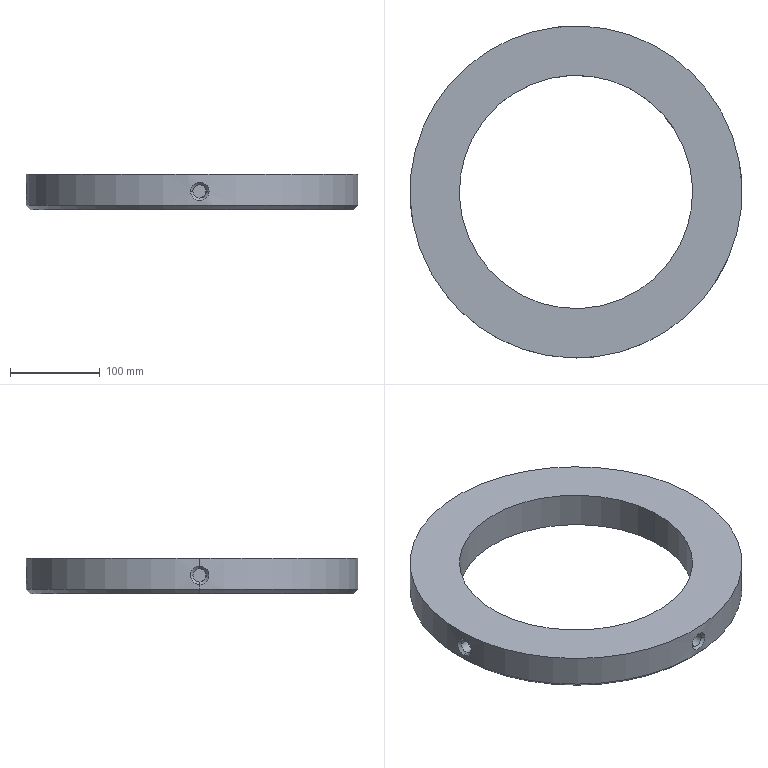Part | SolidWorks | features BaseBody 1 | 1 solid | 32 faces | box 370 x 370 x 40 mm | volume 2151214 mm3 | spline 12 | cylinder 12 | plane 6 | cone 2 | commonest cylinder face diameters 15 x8 260 x2 370 x2